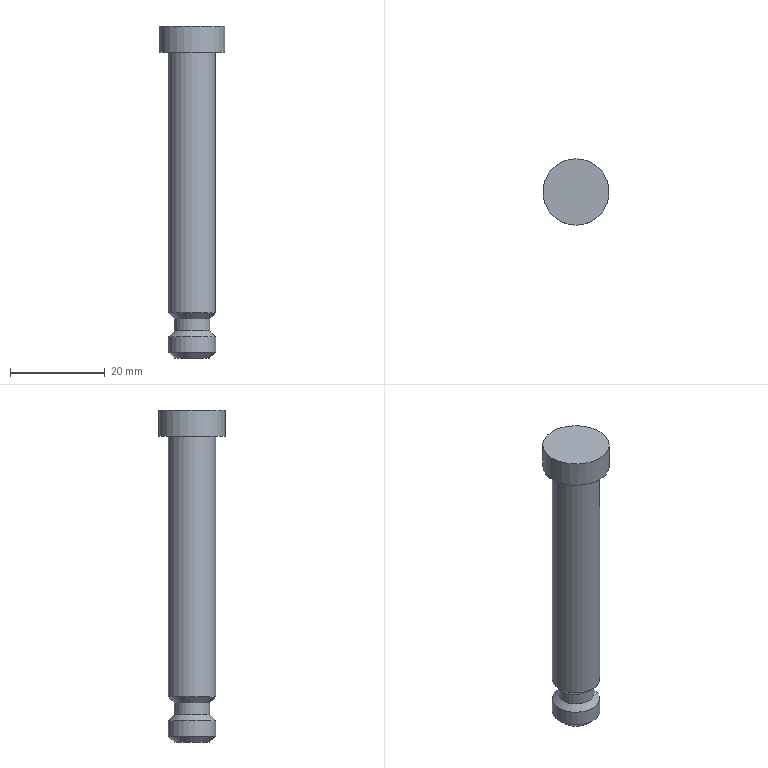Part | NX | features solid 2 | 1 solid | 10 faces | box 14 x 14 x 70 mm | volume 5759 mm3 | cylinder 4 | plane 3 | cone 3 | commonest cylinder face diameters 10 x2 7.5 x1 14 x1
STEP:
#1=CARTESIAN_POINT('',(25.,-440.,-33.75));
#2=VERTEX_POINT('',#1);
#3=CARTESIAN_POINT('',(25.,-435.,-33.75));
#4=DIRECTION('',(0.,0.,-1.));
#5=DIRECTION('',(0.,-1.,0.));
#6=AXIS2_PLACEMENT_3D('',#3,#4,#5);
#7=CIRCLE('',#6,5.);
#8=EDGE_CURVE('',#2,#2,#7,.F.);
#9=ORIENTED_EDGE('',*,*,#8,.T.);
#10=EDGE_LOOP('',(#9));
#11=FACE_BOUND('',#10,.T.);
#12=CARTESIAN_POINT('',(25.,-430.,-30.5));
#13=VERTEX_POINT('',#12);
#14=CARTESIAN_POINT('',(25.,-435.,-30.5));
#15=DIRECTION('',(0.,0.,1.));
#16=DIRECTION('',(0.,1.,0.));
#17=AXIS2_PLACEMENT_3D('',#14,#15,#16);
#18=CIRCLE('',#17,5.);
#19=EDGE_CURVE('',#13,#13,#18,.F.);
#20=ORIENTED_EDGE('',*,*,#19,.T.);
#21=EDGE_LOOP('',(#20));
#22=FACE_BOUND('',#21,.T.);
#23=CARTESIAN_POINT('',(25.,-435.,-35.));
#24=DIRECTION('',(0.,0.,1.));
#25=DIRECTION('',(0.,1.,0.));
#26=AXIS2_PLACEMENT_3D('',#23,#24,#25);
#27=CYLINDRICAL_SURFACE('',#26,5.);
#28=ADVANCED_FACE('',(#11,#22),#27,.T.);
#29=CARTESIAN_POINT('',(25.,-438.75,-35.));
#30=VERTEX_POINT('',#29);
#31=CARTESIAN_POINT('',(25.,-435.,-35.));
#32=DIRECTION('',(0.,0.,-1.));
#33=DIRECTION('',(0.,-1.,0.));
#34=AXIS2_PLACEMENT_3D('',#31,#32,#33);
#35=CIRCLE('',#34,3.75);
#36=EDGE_CURVE('',#30,#30,#35,.T.);
#37=ORIENTED_EDGE('',*,*,#36,.T.);
#38=EDGE_LOOP('',(#37));
#39=FACE_BOUND('',#38,.T.);
#40=CARTESIAN_POINT('',(25.,-435.,-35.));
#41=DIRECTION('',(0.,0.,-1.));
#42=DIRECTION('',(0.,-1.,0.));
#43=AXIS2_PLACEMENT_3D('',#40,#41,#42);
#44=PLANE('',#43);
#45=ADVANCED_FACE('',(#39),#44,.T.);
#46=CARTESIAN_POINT('',(25.,-438.75,-29.25));
#47=VERTEX_POINT('',#46);
#48=CARTESIAN_POINT('',(25.,-435.,-29.25));
#49=DIRECTION('',(0.,0.,-1.));
#50=DIRECTION('',(0.,-1.,0.));
#51=AXIS2_PLACEMENT_3D('',#48,#49,#50);
#52=CIRCLE('',#51,3.75);
#53=EDGE_CURVE('',#47,#47,#52,.T.);
#54=ORIENTED_EDGE('',*,*,#53,.F.);
#55=EDGE_LOOP('',(#54));
#56=FACE_BOUND('',#55,.T.);
#57=CARTESIAN_POINT('',(25.,-438.75,-26.75));
#58=VERTEX_POINT('',#57);
#59=CARTESIAN_POINT('',(25.,-435.,-26.75));
#60=DIRECTION('',(0.,0.,-1.));
#61=DIRECTION('',(0.,-1.,0.));
#62=AXIS2_PLACEMENT_3D('',#59,#60,#61);
#63=CIRCLE('',#62,3.75);
#64=EDGE_CURVE('',#58,#58,#63,.T.);
#65=ORIENTED_EDGE('',*,*,#64,.T.);
#66=EDGE_LOOP('',(#65));
#67=FACE_BOUND('',#66,.T.);
#68=CARTESIAN_POINT('',(25.,-435.,-26.75));
#69=DIRECTION('',(0.,0.,-1.));
#70=DIRECTION('',(0.,-1.,0.));
#71=AXIS2_PLACEMENT_3D('',#68,#69,#70);
#72=CYLINDRICAL_SURFACE('',#71,3.75);
#73=ADVANCED_FACE('',(#56,#67),#72,.T.);
#74=CARTESIAN_POINT('',(25.,-440.,-25.5));
#75=VERTEX_POINT('',#74);
#76=CARTESIAN_POINT('',(25.,-435.,-25.5));
#77=DIRECTION('',(0.,0.,-1.));
#78=DIRECTION('',(0.,-1.,0.));
#79=AXIS2_PLACEMENT_3D('',#76,#77,#78);
#80=CIRCLE('',#79,5.);
#81=EDGE_CURVE('',#75,#75,#80,.F.);
#82=ORIENTED_EDGE('',*,*,#81,.T.);
#83=EDGE_LOOP('',(#82));
#84=FACE_BOUND('',#83,.T.);
#85=CARTESIAN_POINT('',(25.,-440.,29.5));
#86=VERTEX_POINT('',#85);
#87=CARTESIAN_POINT('',(25.,-435.,29.5));
#88=DIRECTION('',(0.,0.,-1.));
#89=DIRECTION('',(0.,-1.,0.));
#90=AXIS2_PLACEMENT_3D('',#87,#88,#89);
#91=CIRCLE('',#90,5.);
#92=EDGE_CURVE('',#86,#86,#91,.T.);
#93=ORIENTED_EDGE('',*,*,#92,.T.);
#94=EDGE_LOOP('',(#93));
#95=FACE_BOUND('',#94,.T.);
#96=CARTESIAN_POINT('',(25.,-435.,-35.));
#97=DIRECTION('',(0.,0.,1.));
#98=DIRECTION('',(0.,1.,0.));
#99=AXIS2_PLACEMENT_3D('',#96,#97,#98);
#100=CYLINDRICAL_SURFACE('',#99,5.);
#101=ADVANCED_FACE('',(#84,#95),#100,.T.);
#102=ORIENTED_EDGE('',*,*,#53,.T.);
#103=EDGE_LOOP('',(#102));
#104=FACE_BOUND('',#103,.T.);
#105=ORIENTED_EDGE('',*,*,#19,.F.);
#106=EDGE_LOOP('',(#105));
#107=FACE_BOUND('',#106,.T.);
#108=CARTESIAN_POINT('',(25.,-435.,-30.5));
#109=DIRECTION('',(0.,0.,-1.));
#110=DIRECTION('',(0.,-1.,0.));
#111=AXIS2_PLACEMENT_3D('',#108,#109,#110);
#112=CONICAL_SURFACE('',#111,5.,0.7854);
#113=ADVANCED_FACE('',(#104,#107),#112,.T.);
#114=ORIENTED_EDGE('',*,*,#81,.F.);
#115=EDGE_LOOP('',(#114));
#116=FACE_BOUND('',#115,.T.);
#117=ORIENTED_EDGE('',*,*,#64,.F.);
#118=EDGE_LOOP('',(#117));
#119=FACE_BOUND('',#118,.T.);
#120=CARTESIAN_POINT('',(25.,-435.,-26.75));
#121=DIRECTION('',(0.,0.,1.));
#122=DIRECTION('',(0.,1.,0.));
#123=AXIS2_PLACEMENT_3D('',#120,#121,#122);
#124=CONICAL_SURFACE('',#123,3.75,0.7854);
#125=ADVANCED_FACE('',(#116,#119),#124,.T.);
#126=ORIENTED_EDGE('',*,*,#8,.F.);
#127=EDGE_LOOP('',(#126));
#128=FACE_BOUND('',#127,.T.);
#129=ORIENTED_EDGE('',*,*,#36,.F.);
#130=EDGE_LOOP('',(#129));
#131=FACE_BOUND('',#130,.T.);
#132=CARTESIAN_POINT('',(25.,-435.,-35.));
#133=DIRECTION('',(0.,0.,1.));
#134=DIRECTION('',(0.,1.,0.));
#135=AXIS2_PLACEMENT_3D('',#132,#133,#134);
#136=CONICAL_SURFACE('',#135,3.75,0.7854);
#137=ADVANCED_FACE('',(#128,#131),#136,.T.);
#138=CARTESIAN_POINT('',(25.,-442.,29.5));
#139=VERTEX_POINT('',#138);
#140=CARTESIAN_POINT('',(25.,-435.,29.5));
#141=DIRECTION('',(0.,0.,-1.));
#142=DIRECTION('',(0.,-1.,0.));
#143=AXIS2_PLACEMENT_3D('',#140,#141,#142);
#144=CIRCLE('',#143,7.);
#145=EDGE_CURVE('',#139,#139,#144,.T.);
#146=ORIENTED_EDGE('',*,*,#145,.T.);
#147=EDGE_LOOP('',(#146));
#148=FACE_BOUND('',#147,.T.);
#149=ORIENTED_EDGE('',*,*,#92,.F.);
#150=EDGE_LOOP('',(#149));
#151=FACE_BOUND('',#150,.T.);
#152=CARTESIAN_POINT('',(25.,-435.,29.5));
#153=DIRECTION('',(0.,0.,-1.));
#154=DIRECTION('',(0.,-1.,0.));
#155=AXIS2_PLACEMENT_3D('',#152,#153,#154);
#156=PLANE('',#155);
#157=ADVANCED_FACE('',(#148,#151),#156,.T.);
#158=CARTESIAN_POINT('',(25.,-442.,35.));
#159=VERTEX_POINT('',#158);
#160=CARTESIAN_POINT('',(25.,-435.,35.));
#161=DIRECTION('',(0.,0.,-1.));
#162=DIRECTION('',(0.,-1.,0.));
#163=AXIS2_PLACEMENT_3D('',#160,#161,#162);
#164=CIRCLE('',#163,7.);
#165=EDGE_CURVE('',#159,#159,#164,.T.);
#166=ORIENTED_EDGE('',*,*,#165,.T.);
#167=EDGE_LOOP('',(#166));
#168=FACE_BOUND('',#167,.T.);
#169=ORIENTED_EDGE('',*,*,#145,.F.);
#170=EDGE_LOOP('',(#169));
#171=FACE_BOUND('',#170,.T.);
#172=CARTESIAN_POINT('',(25.,-435.,35.));
#173=DIRECTION('',(0.,0.,-1.));
#174=DIRECTION('',(0.,-1.,0.));
#175=AXIS2_PLACEMENT_3D('',#172,#173,#174);
#176=CYLINDRICAL_SURFACE('',#175,7.);
#177=ADVANCED_FACE('',(#168,#171),#176,.T.);
#178=ORIENTED_EDGE('',*,*,#165,.F.);
#179=EDGE_LOOP('',(#178));
#180=FACE_BOUND('',#179,.T.);
#181=CARTESIAN_POINT('',(25.,-435.,35.));
#182=DIRECTION('',(0.,0.,-1.));
#183=DIRECTION('',(0.,-1.,0.));
#184=AXIS2_PLACEMENT_3D('',#181,#182,#183);
#185=PLANE('',#184);
#186=ADVANCED_FACE('',(#180),#185,.F.);
#187=CLOSED_SHELL('',(#28,#45,#73,#101,#113,#125,#137,#157,#177,#186));
#188=MANIFOLD_SOLID_BREP('',#187);
#189=(LENGTH_UNIT()NAMED_UNIT(*)SI_UNIT(.MILLI.,.METRE.));
#190=UNCERTAINTY_MEASURE_WITH_UNIT(LENGTH_MEASURE(0.00001),#189,'','');
#191=(NAMED_UNIT(*)PLANE_ANGLE_UNIT()SI_UNIT($,.RADIAN.));
#192=(NAMED_UNIT(*)SI_UNIT($,.STERADIAN.)SOLID_ANGLE_UNIT());
#193=(GEOMETRIC_REPRESENTATION_CONTEXT(3)GLOBAL_UNCERTAINTY_ASSIGNED_CONTEXT((#190))GLOBAL_UNIT_ASSIGNED_CONTEXT((#189,#191,#192))REPRESENTATION_CONTEXT('',''));
#194=ADVANCED_BREP_SHAPE_REPRESENTATION('',(#188),#193);